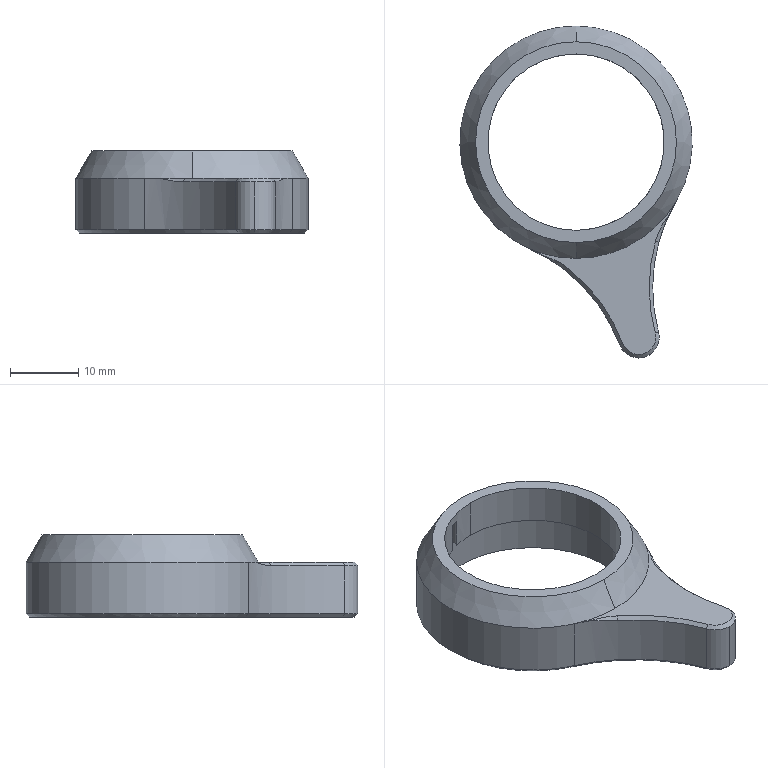Part | SolidWorks | features BaseBody 1 | 1 solid | 35 faces | box 34 x 48.563 x 12 mm | volume 4249 mm3 | cone 16 | cylinder 14 | plane 5 | commonest cylinder face diameters 2.5 x3 29.5 x3 6 x2 25.8 x2 34 x2 50 x2
STEP:
#1=CARTESIAN_POINT('',(599.943,-176.052,243.045));
#2=VERTEX_POINT('',#1);
#3=CARTESIAN_POINT('',(593.042,-208.588,243.045));
#4=VERTEX_POINT('',#3);
#5=CARTESIAN_POINT('',(599.943,-193.052,243.045));
#6=DIRECTION('',(0.000000001,-0.000000003,1.));
#7=DIRECTION('',(0.3057,-0.9521,-0.000000003));
#8=AXIS2_PLACEMENT_3D('',#5,#6,#7);
#9=CIRCLE('',#8,17.);
#10=EDGE_CURVE('',#2,#4,#9,.T.);
#11=ORIENTED_EDGE('',*,*,#10,.F.);
#12=CARTESIAN_POINT('',(599.943,-176.052,235.545));
#13=VERTEX_POINT('',#12);
#14=CARTESIAN_POINT('',(599.943,-176.052,243.045));
#15=DIRECTION('',(-0.000000001,0.000000003,-1.));
#16=VECTOR('',#15,1000.);
#17=LINE('',#14,#16);
#18=EDGE_CURVE('',#2,#13,#17,.T.);
#19=ORIENTED_EDGE('',*,*,#18,.T.);
#20=CARTESIAN_POINT('',(593.042,-208.588,235.545));
#21=VERTEX_POINT('',#20);
#22=CARTESIAN_POINT('',(599.943,-193.052,235.545));
#23=DIRECTION('',(-0.000000001,0.000000003,-1.));
#24=DIRECTION('',(0.3057,-0.9521,-0.000000003));
#25=AXIS2_PLACEMENT_3D('',#22,#23,#24);
#26=CIRCLE('',#25,17.);
#27=EDGE_CURVE('',#21,#13,#26,.T.);
#28=ORIENTED_EDGE('',*,*,#27,.F.);
#29=CARTESIAN_POINT('',(593.042,-208.588,239.295));
#30=DIRECTION('',(-0.000000001,0.000000003,-1.));
#31=VECTOR('',#30,1000.);
#32=LINE('',#29,#31);
#33=EDGE_CURVE('',#4,#21,#32,.T.);
#34=ORIENTED_EDGE('',*,*,#33,.F.);
#35=EDGE_LOOP('',(#11,#19,#28,#34));
#36=FACE_OUTER_BOUND('',#35,.T.);
#37=CARTESIAN_POINT('',(599.943,-193.052,243.045));
#38=DIRECTION('',(-0.000000001,0.000000003,-1.));
#39=DIRECTION('',(0.,1.,0.000000003));
#40=AXIS2_PLACEMENT_3D('',#37,#38,#39);
#41=CYLINDRICAL_SURFACE('',#40,17.);
#42=ADVANCED_FACE('',(#36),#41,.T.);
#43=CARTESIAN_POINT('',(599.943,-207.742,247.045));
#44=VERTEX_POINT('',#43);
#45=CARTESIAN_POINT('',(599.943,-178.361,247.045));
#46=VERTEX_POINT('',#45);
#47=CARTESIAN_POINT('',(599.943,-193.052,247.045));
#48=DIRECTION('',(0.000000001,-0.000000003,1.));
#49=DIRECTION('',(0.,1.,0.000000003));
#50=AXIS2_PLACEMENT_3D('',#47,#48,#49);
#51=CIRCLE('',#50,14.691);
#52=EDGE_CURVE('',#44,#46,#51,.T.);
#53=ORIENTED_EDGE('',*,*,#52,.F.);
#54=CARTESIAN_POINT('',(599.943,-210.052,243.045));
#55=VERTEX_POINT('',#54);
#56=CARTESIAN_POINT('',(599.943,-207.742,247.045));
#57=DIRECTION('',(-0.000000001,-0.5,-0.866));
#58=VECTOR('',#57,1000.);
#59=LINE('',#56,#58);
#60=EDGE_CURVE('',#44,#55,#59,.T.);
#61=ORIENTED_EDGE('',*,*,#60,.T.);
#62=CARTESIAN_POINT('',(614.599,-201.666,243.045));
#63=VERTEX_POINT('',#62);
#64=CARTESIAN_POINT('',(599.943,-193.052,243.045));
#65=DIRECTION('',(-0.000000001,0.000000003,-1.));
#66=DIRECTION('',(0.,1.,0.000000003));
#67=AXIS2_PLACEMENT_3D('',#64,#65,#66);
#68=CIRCLE('',#67,17.);
#69=EDGE_CURVE('',#63,#55,#68,.T.);
#70=ORIENTED_EDGE('',*,*,#69,.F.);
#71=CARTESIAN_POINT('',(599.943,-193.052,243.045));
#72=DIRECTION('',(0.000000001,-0.000000003,1.));
#73=DIRECTION('',(0.3057,-0.9521,-0.000000003));
#74=AXIS2_PLACEMENT_3D('',#71,#72,#73);
#75=CIRCLE('',#74,17.);
#76=EDGE_CURVE('',#63,#2,#75,.T.);
#77=ORIENTED_EDGE('',*,*,#76,.T.);
#78=CARTESIAN_POINT('',(599.943,-178.361,247.045));
#79=DIRECTION('',(-0.000000001,0.5,-0.866));
#80=VECTOR('',#79,1000.);
#81=LINE('',#78,#80);
#82=EDGE_CURVE('',#46,#2,#81,.T.);
#83=ORIENTED_EDGE('',*,*,#82,.F.);
#84=EDGE_LOOP('',(#53,#61,#70,#77,#83));
#85=FACE_OUTER_BOUND('',#84,.T.);
#86=CARTESIAN_POINT('',(599.943,-193.052,247.045));
#87=DIRECTION('',(-0.000000001,0.000000003,-1.));
#88=DIRECTION('',(0.,1.,0.000000003));
#89=AXIS2_PLACEMENT_3D('',#86,#87,#88);
#90=CONICAL_SURFACE('',#89,14.691,0.5236);
#91=ADVANCED_FACE('',(#85),#90,.T.);
#92=CARTESIAN_POINT('',(609.115,-224.615,235.545));
#93=VERTEX_POINT('',#92);
#94=CARTESIAN_POINT('',(606.305,-222.667,235.545));
#95=VERTEX_POINT('',#94);
#96=CARTESIAN_POINT('',(609.115,-221.615,235.545));
#97=DIRECTION('',(-0.000000001,0.000000003,-1.));
#98=DIRECTION('',(0.3057,-0.9521,-0.000000003));
#99=AXIS2_PLACEMENT_3D('',#96,#97,#98);
#100=CIRCLE('',#99,3.);
#101=EDGE_CURVE('',#93,#95,#100,.T.);
#102=ORIENTED_EDGE('',*,*,#101,.F.);
#103=CARTESIAN_POINT('',(609.115,-224.615,242.545));
#104=VERTEX_POINT('',#103);
#105=CARTESIAN_POINT('',(609.115,-224.615,235.545));
#106=DIRECTION('',(0.000000001,-0.000000003,1.));
#107=VECTOR('',#106,1000.);
#108=LINE('',#105,#107);
#109=EDGE_CURVE('',#93,#104,#108,.T.);
#110=ORIENTED_EDGE('',*,*,#109,.T.);
#111=CARTESIAN_POINT('',(606.305,-222.667,242.545));
#112=VERTEX_POINT('',#111);
#113=CARTESIAN_POINT('',(609.115,-221.615,242.545));
#114=DIRECTION('',(0.000000001,-0.000000003,1.));
#115=DIRECTION('',(0.3057,-0.9521,-0.000000003));
#116=AXIS2_PLACEMENT_3D('',#113,#114,#115);
#117=CIRCLE('',#116,3.);
#118=EDGE_CURVE('',#112,#104,#117,.T.);
#119=ORIENTED_EDGE('',*,*,#118,.F.);
#120=CARTESIAN_POINT('',(606.305,-222.667,239.295));
#121=DIRECTION('',(0.000000001,-0.000000003,1.));
#122=VECTOR('',#121,1000.);
#123=LINE('',#120,#122);
#124=EDGE_CURVE('',#95,#112,#123,.T.);
#125=ORIENTED_EDGE('',*,*,#124,.F.);
#126=EDGE_LOOP('',(#102,#110,#119,#125));
#127=FACE_OUTER_BOUND('',#126,.T.);
#128=CARTESIAN_POINT('',(609.115,-221.615,235.545));
#129=DIRECTION('',(0.000000001,-0.000000003,1.));
#130=DIRECTION('',(0.,-1.,-0.000000003));
#131=AXIS2_PLACEMENT_3D('',#128,#129,#130);
#132=CYLINDRICAL_SURFACE('',#131,3.);
#133=ADVANCED_FACE('',(#127),#132,.T.);
#134=CARTESIAN_POINT('',(599.943,-207.802,235.045));
#135=VERTEX_POINT('',#134);
#136=CARTESIAN_POINT('',(603.545,-207.355,235.045));
#137=VERTEX_POINT('',#136);
#138=CARTESIAN_POINT('',(599.943,-193.052,235.045));
#139=DIRECTION('',(0.000000001,-0.000000003,1.));
#140=DIRECTION('',(0.,-1.,-0.000000003));
#141=AXIS2_PLACEMENT_3D('',#138,#139,#140);
#142=CIRCLE('',#141,14.75);
#143=EDGE_CURVE('',#135,#137,#142,.T.);
#144=ORIENTED_EDGE('',*,*,#143,.F.);
#145=CARTESIAN_POINT('',(599.943,-207.802,241.245));
#146=VERTEX_POINT('',#145);
#147=CARTESIAN_POINT('',(599.943,-207.802,235.045));
#148=DIRECTION('',(0.000000001,-0.000000003,1.));
#149=VECTOR('',#148,1000.);
#150=LINE('',#147,#149);
#151=EDGE_CURVE('',#135,#146,#150,.T.);
#152=ORIENTED_EDGE('',*,*,#151,.T.);
#153=CARTESIAN_POINT('',(603.545,-207.355,241.245));
#154=VERTEX_POINT('',#153);
#155=CARTESIAN_POINT('',(599.943,-193.052,241.245));
#156=DIRECTION('',(0.000000001,-0.000000003,1.));
#157=DIRECTION('',(0.,-1.,-0.000000003));
#158=AXIS2_PLACEMENT_3D('',#155,#156,#157);
#159=CIRCLE('',#158,14.75);
#160=EDGE_CURVE('',#146,#154,#159,.T.);
#161=ORIENTED_EDGE('',*,*,#160,.T.);
#162=CARTESIAN_POINT('',(603.545,-207.355,238.145));
#163=DIRECTION('',(-0.000000001,0.000000003,-1.));
#164=VECTOR('',#163,1000.);
#165=LINE('',#162,#164);
#166=EDGE_CURVE('',#154,#137,#165,.T.);
#167=ORIENTED_EDGE('',*,*,#166,.T.);
#168=EDGE_LOOP('',(#144,#152,#161,#167));
#169=FACE_OUTER_BOUND('',#168,.T.);
#170=CARTESIAN_POINT('',(599.943,-193.052,235.045));
#171=DIRECTION('',(0.000000001,-0.000000003,1.));
#172=DIRECTION('',(0.,-1.,-0.000000003));
#173=AXIS2_PLACEMENT_3D('',#170,#171,#172);
#174=CYLINDRICAL_SURFACE('',#173,14.75);
#175=ADVANCED_FACE('',(#169),#174,.F.);
#176=CARTESIAN_POINT('',(609.115,-224.115,235.045));
#177=VERTEX_POINT('',#176);
#178=CARTESIAN_POINT('',(606.774,-222.492,235.045));
#179=VERTEX_POINT('',#178);
#180=CARTESIAN_POINT('',(609.115,-221.615,235.045));
#181=DIRECTION('',(-0.000000001,0.000000003,-1.));
#182=DIRECTION('',(0.,-1.,-0.000000003));
#183=AXIS2_PLACEMENT_3D('',#180,#181,#182);
#184=CIRCLE('',#183,2.5);
#185=EDGE_CURVE('',#177,#179,#184,.T.);
#186=ORIENTED_EDGE('',*,*,#185,.F.);
#187=CARTESIAN_POINT('',(609.115,-224.115,235.045));
#188=DIRECTION('',(0.000000001,-0.7071,0.7071));
#189=VECTOR('',#188,1000.);
#190=LINE('',#187,#189);
#191=EDGE_CURVE('',#177,#93,#190,.T.);
#192=ORIENTED_EDGE('',*,*,#191,.T.);
#193=ORIENTED_EDGE('',*,*,#101,.T.);
#194=CARTESIAN_POINT('',(606.539,-222.58,235.295));
#195=DIRECTION('',(-0.6622,-0.248,0.7071));
#196=VECTOR('',#195,1000.);
#197=LINE('',#194,#196);
#198=EDGE_CURVE('',#179,#95,#197,.T.);
#199=ORIENTED_EDGE('',*,*,#198,.F.);
#200=EDGE_LOOP('',(#186,#192,#193,#199));
#201=FACE_OUTER_BOUND('',#200,.T.);
#202=CARTESIAN_POINT('',(609.115,-221.615,235.045));
#203=DIRECTION('',(0.000000001,-0.000000003,1.));
#204=DIRECTION('',(0.,-1.,-0.000000003));
#205=AXIS2_PLACEMENT_3D('',#202,#203,#204);
#206=CONICAL_SURFACE('',#205,2.5,0.7854);
#207=ADVANCED_FACE('',(#201),#206,.T.);
#208=CARTESIAN_POINT('',(599.943,-180.152,247.045));
#209=VERTEX_POINT('',#208);
#210=CARTESIAN_POINT('',(599.943,-205.952,247.045));
#211=VERTEX_POINT('',#210);
#212=CARTESIAN_POINT('',(599.943,-193.052,247.045));
#213=DIRECTION('',(0.000000001,-0.000000003,1.));
#214=DIRECTION('',(0.,1.,0.000000003));
#215=AXIS2_PLACEMENT_3D('',#212,#213,#214);
#216=CIRCLE('',#215,12.9);
#217=EDGE_CURVE('',#209,#211,#216,.T.);
#218=ORIENTED_EDGE('',*,*,#217,.T.);
#219=CARTESIAN_POINT('',(599.943,-205.952,241.245));
#220=VERTEX_POINT('',#219);
#221=CARTESIAN_POINT('',(599.943,-205.952,247.045));
#222=DIRECTION('',(-0.000000001,0.000000003,-1.));
#223=VECTOR('',#222,1000.);
#224=LINE('',#221,#223);
#225=EDGE_CURVE('',#211,#220,#224,.T.);
#226=ORIENTED_EDGE('',*,*,#225,.T.);
#227=CARTESIAN_POINT('',(595.317,-181.009,241.245));
#228=VERTEX_POINT('',#227);
#229=CARTESIAN_POINT('',(599.943,-193.052,241.245));
#230=DIRECTION('',(-0.000000001,0.000000003,-1.));
#231=DIRECTION('',(0.,1.,0.000000003));
#232=AXIS2_PLACEMENT_3D('',#229,#230,#231);
#233=CIRCLE('',#232,12.9);
#234=EDGE_CURVE('',#220,#228,#233,.T.);
#235=ORIENTED_EDGE('',*,*,#234,.T.);
#236=CARTESIAN_POINT('',(595.317,-181.009,245.545));
#237=VERTEX_POINT('',#236);
#238=CARTESIAN_POINT('',(595.317,-181.009,244.145));
#239=DIRECTION('',(0.000000001,-0.000000003,1.));
#240=VECTOR('',#239,1000.);
#241=LINE('',#238,#240);
#242=EDGE_CURVE('',#228,#237,#241,.T.);
#243=ORIENTED_EDGE('',*,*,#242,.T.);
#244=CARTESIAN_POINT('',(595.693,-180.872,245.657));
#245=VERTEX_POINT('',#244);
#246=CARTESIAN_POINT('',(595.693,-180.872,245.657));
#247=CARTESIAN_POINT('',(595.565,-180.916,245.632));
#248=CARTESIAN_POINT('',(595.439,-180.962,245.592));
#249=CARTESIAN_POINT('',(595.317,-181.009,245.545));
#250=B_SPLINE_CURVE_WITH_KNOTS('',3,(#246,#247,#248,#249),.UNSPECIFIED.,.F.,.F.,(4,4),(0.001058,0.001468),.UNSPECIFIED.);
#251=EDGE_CURVE('',#245,#237,#250,.T.);
#252=ORIENTED_EDGE('',*,*,#251,.F.);
#253=CARTESIAN_POINT('',(596.693,-180.568,245.545));
#254=VERTEX_POINT('',#253);
#255=CARTESIAN_POINT('',(596.693,-180.568,245.545));
#256=CARTESIAN_POINT('',(596.53,-180.61,245.605));
#257=CARTESIAN_POINT('',(596.366,-180.656,245.653));
#258=CARTESIAN_POINT('',(596.031,-180.758,245.698));
#259=CARTESIAN_POINT('',(595.858,-180.814,245.691));
#260=CARTESIAN_POINT('',(595.693,-180.872,245.657));
#261=B_SPLINE_CURVE_WITH_KNOTS('',3,(#255,#256,#257,#258,#259,#260),.UNSPECIFIED.,.F.,.F.,(4,2,4),(0.,0.0005289,0.001058),.UNSPECIFIED.);
#262=EDGE_CURVE('',#254,#245,#261,.T.);
#263=ORIENTED_EDGE('',*,*,#262,.F.);
#264=CARTESIAN_POINT('',(596.693,-180.568,241.245));
#265=VERTEX_POINT('',#264);
#266=CARTESIAN_POINT('',(596.693,-180.568,244.145));
#267=DIRECTION('',(-0.000000001,0.000000003,-1.));
#268=VECTOR('',#267,1000.);
#269=LINE('',#266,#268);
#270=EDGE_CURVE('',#254,#265,#269,.T.);
#271=ORIENTED_EDGE('',*,*,#270,.T.);
#272=CARTESIAN_POINT('',(599.943,-180.152,241.245));
#273=VERTEX_POINT('',#272);
#274=CARTESIAN_POINT('',(599.943,-193.052,241.245));
#275=DIRECTION('',(-0.000000001,0.000000003,-1.));
#276=DIRECTION('',(0.,1.,0.000000003));
#277=AXIS2_PLACEMENT_3D('',#274,#275,#276);
#278=CIRCLE('',#277,12.9);
#279=EDGE_CURVE('',#265,#273,#278,.T.);
#280=ORIENTED_EDGE('',*,*,#279,.T.);
#281=CARTESIAN_POINT('',(599.943,-180.152,247.045));
#282=DIRECTION('',(-0.000000001,0.000000003,-1.));
#283=VECTOR('',#282,1000.);
#284=LINE('',#281,#283);
#285=EDGE_CURVE('',#209,#273,#284,.T.);
#286=ORIENTED_EDGE('',*,*,#285,.F.);
#287=EDGE_LOOP('',(#218,#226,#235,#243,#252,#263,#271,#280,#286));
#288=FACE_OUTER_BOUND('',#287,.T.);
#289=CARTESIAN_POINT('',(599.943,-193.052,247.045));
#290=DIRECTION('',(-0.000000001,0.000000003,-1.));
#291=DIRECTION('',(0.,1.,0.000000003));
#292=AXIS2_PLACEMENT_3D('',#289,#290,#291);
#293=CYLINDRICAL_SURFACE('',#292,12.9);
#294=ADVANCED_FACE('',(#288),#293,.F.);
#295=CARTESIAN_POINT('',(595.693,-178.567,245.545));
#296=VERTEX_POINT('',#295);
#297=CARTESIAN_POINT('',(595.693,-179.817,245.545));
#298=DIRECTION('',(0.000000001,-0.000000003,1.));
#299=DIRECTION('',(0.3057,-0.9521,-0.000000003));
#300=AXIS2_PLACEMENT_3D('',#297,#298,#299);
#301=CIRCLE('',#300,1.25);
#302=EDGE_CURVE('',#254,#296,#301,.T.);
#303=ORIENTED_EDGE('',*,*,#302,.T.);
#304=CARTESIAN_POINT('',(595.693,-178.567,235.045));
#305=VERTEX_POINT('',#304);
#306=CARTESIAN_POINT('',(595.693,-178.567,245.545));
#307=DIRECTION('',(-0.000000001,0.000000003,-1.));
#308=VECTOR('',#307,1000.);
#309=LINE('',#306,#308);
#310=EDGE_CURVE('',#296,#305,#309,.T.);
#311=ORIENTED_EDGE('',*,*,#310,.T.);
#312=CARTESIAN_POINT('',(596.341,-178.748,235.045));
#313=VERTEX_POINT('',#312);
#314=CARTESIAN_POINT('',(595.693,-179.817,235.045));
#315=DIRECTION('',(-0.000000001,0.000000003,-1.));
#316=DIRECTION('',(0.,1.,0.000000003));
#317=AXIS2_PLACEMENT_3D('',#314,#315,#316);
#318=CIRCLE('',#317,1.25);
#319=EDGE_CURVE('',#305,#313,#318,.T.);
#320=ORIENTED_EDGE('',*,*,#319,.T.);
#321=CARTESIAN_POINT('',(596.341,-178.748,241.245));
#322=VERTEX_POINT('',#321);
#323=CARTESIAN_POINT('',(596.341,-178.748,238.145));
#324=DIRECTION('',(-0.000000001,0.000000003,-1.));
#325=VECTOR('',#324,1000.);
#326=LINE('',#323,#325);
#327=EDGE_CURVE('',#322,#313,#326,.T.);
#328=ORIENTED_EDGE('',*,*,#327,.F.);
#329=CARTESIAN_POINT('',(595.693,-179.817,241.245));
#330=DIRECTION('',(-0.000000001,0.000000003,-1.));
#331=DIRECTION('',(0.,1.,0.000000003));
#332=AXIS2_PLACEMENT_3D('',#329,#330,#331);
#333=CIRCLE('',#332,1.25);
#334=EDGE_CURVE('',#322,#265,#333,.T.);
#335=ORIENTED_EDGE('',*,*,#334,.T.);
#336=ORIENTED_EDGE('',*,*,#270,.F.);
#337=EDGE_LOOP('',(#303,#311,#320,#328,#335,#336));
#338=FACE_OUTER_BOUND('',#337,.T.);
#339=CARTESIAN_POINT('',(595.693,-179.817,245.545));
#340=DIRECTION('',(-0.000000001,0.000000003,-1.));
#341=DIRECTION('',(0.,1.,0.000000003));
#342=AXIS2_PLACEMENT_3D('',#339,#340,#341);
#343=CYLINDRICAL_SURFACE('',#342,1.25);
#344=ADVANCED_FACE('',(#338),#343,.F.);
#345=CARTESIAN_POINT('',(604.192,-206.286,246.266));
#346=VERTEX_POINT('',#345);
#347=CARTESIAN_POINT('',(604.192,-205.231,245.657));
#348=VERTEX_POINT('',#347);
#349=CARTESIAN_POINT('',(604.192,-206.286,246.266));
#350=DIRECTION('',(0.,0.866,-0.5));
#351=VECTOR('',#350,1000.);
#352=LINE('',#349,#351);
#353=EDGE_CURVE('',#346,#348,#352,.T.);
#354=ORIENTED_EDGE('',*,*,#353,.F.);
#355=CARTESIAN_POINT('',(604.192,-207.536,245.545));
#356=VERTEX_POINT('',#355);
#357=CARTESIAN_POINT('',(604.192,-206.286,246.266));
#358=DIRECTION('',(0.,-0.866,-0.5));
#359=VECTOR('',#358,1000.);
#360=LINE('',#357,#359);
#361=EDGE_CURVE('',#346,#356,#360,.T.);
#362=ORIENTED_EDGE('',*,*,#361,.T.);
#363=CARTESIAN_POINT('',(603.193,-205.535,245.545));
#364=VERTEX_POINT('',#363);
#365=CARTESIAN_POINT('',(604.192,-206.286,245.545));
#366=DIRECTION('',(0.000000001,-0.000000003,1.));
#367=DIRECTION('',(0.3057,-0.9521,-0.000000003));
#368=AXIS2_PLACEMENT_3D('',#365,#366,#367);
#369=CIRCLE('',#368,1.25);
#370=EDGE_CURVE('',#364,#356,#369,.T.);
#371=ORIENTED_EDGE('',*,*,#370,.F.);
#372=CARTESIAN_POINT('',(603.193,-205.535,245.545));
#373=CARTESIAN_POINT('',(603.355,-205.493,245.605));
#374=CARTESIAN_POINT('',(603.519,-205.447,245.653));
#375=CARTESIAN_POINT('',(603.855,-205.345,245.698));
#376=CARTESIAN_POINT('',(604.028,-205.289,245.691));
#377=CARTESIAN_POINT('',(604.192,-205.231,245.657));
#378=B_SPLINE_CURVE_WITH_KNOTS('',3,(#372,#373,#374,#375,#376,#377),.UNSPECIFIED.,.F.,.F.,(4,2,4),(-0.0007426,-0.0002096,0.0003234),.UNSPECIFIED.);
#379=EDGE_CURVE('',#364,#348,#378,.T.);
#380=ORIENTED_EDGE('',*,*,#379,.T.);
#381=EDGE_LOOP('',(#354,#362,#371,#380));
#382=FACE_OUTER_BOUND('',#381,.T.);
#383=CARTESIAN_POINT('',(604.192,-206.286,-753.734));
#384=DIRECTION('',(-0.000000001,0.000000003,-1.));
#385=DIRECTION('',(0.,1.,0.000000003));
#386=AXIS2_PLACEMENT_3D('',#383,#384,#385);
#387=CONICAL_SURFACE('',#386,1732.051,1.047);
#388=ADVANCED_FACE('',(#382),#387,.F.);
#389=CARTESIAN_POINT('',(595.693,-179.817,246.266));
#390=VERTEX_POINT('',#389);
#391=CARTESIAN_POINT('',(595.693,-179.817,246.266));
#392=DIRECTION('',(0.,0.866,-0.5));
#393=VECTOR('',#392,1000.);
#394=LINE('',#391,#393);
#395=EDGE_CURVE('',#390,#296,#394,.T.);
#396=ORIENTED_EDGE('',*,*,#395,.F.);
#397=CARTESIAN_POINT('',(595.693,-179.817,246.266));
#398=DIRECTION('',(0.,-0.866,-0.5));
#399=VECTOR('',#398,1000.);
#400=LINE('',#397,#399);
#401=EDGE_CURVE('',#390,#245,#400,.T.);
#402=ORIENTED_EDGE('',*,*,#401,.T.);
#403=ORIENTED_EDGE('',*,*,#251,.T.);
#404=CARTESIAN_POINT('',(595.693,-179.817,245.545));
#405=DIRECTION('',(0.000000001,-0.000000003,1.));
#406=DIRECTION('',(0.3057,-0.9521,-0.000000003));
#407=AXIS2_PLACEMENT_3D('',#404,#405,#406);
#408=CIRCLE('',#407,1.25);
#409=EDGE_CURVE('',#296,#237,#408,.T.);
#410=ORIENTED_EDGE('',*,*,#409,.F.);
#411=EDGE_LOOP('',(#396,#402,#403,#410));
#412=FACE_OUTER_BOUND('',#411,.T.);
#413=CARTESIAN_POINT('',(595.693,-179.817,-753.734));
#414=DIRECTION('',(-0.000000001,0.000000003,-1.));
#415=DIRECTION('',(0.,1.,0.000000003));
#416=AXIS2_PLACEMENT_3D('',#413,#414,#415);
#417=CONICAL_SURFACE('',#416,1732.051,1.047);
#418=ADVANCED_FACE('',(#412),#417,.F.);
#419=ORIENTED_EDGE('',*,*,#18,.F.);
#420=ORIENTED_EDGE('',*,*,#76,.F.);
#421=CARTESIAN_POINT('',(614.599,-201.666,235.545));
#422=VERTEX_POINT('',#421);
#423=CARTESIAN_POINT('',(614.599,-201.666,239.295));
#424=DIRECTION('',(0.000000001,-0.000000003,1.));
#425=VECTOR('',#424,1000.);
#426=LINE('',#423,#425);
#427=EDGE_CURVE('',#422,#63,#426,.T.);
#428=ORIENTED_EDGE('',*,*,#427,.F.);
#429=CARTESIAN_POINT('',(599.943,-193.052,235.545));
#430=DIRECTION('',(-0.000000001,0.000000003,-1.));
#431=DIRECTION('',(0.3057,-0.9521,-0.000000003));
#432=AXIS2_PLACEMENT_3D('',#429,#430,#431);
#433=CIRCLE('',#432,17.);
#434=EDGE_CURVE('',#13,#422,#433,.T.);
#435=ORIENTED_EDGE('',*,*,#434,.F.);
#436=EDGE_LOOP('',(#419,#420,#428,#435));
#437=FACE_OUTER_BOUND('',#436,.T.);
#438=CARTESIAN_POINT('',(599.943,-193.052,243.045));
#439=DIRECTION('',(-0.000000001,0.000000003,-1.));
#440=DIRECTION('',(0.,1.,0.000000003));
#441=AXIS2_PLACEMENT_3D('',#438,#439,#440);
#442=CYLINDRICAL_SURFACE('',#441,17.);
#443=ADVANCED_FACE('',(#437),#442,.T.);
#444=CARTESIAN_POINT('',(593.245,-208.131,235.045));
#445=VERTEX_POINT('',#444);
#446=CARTESIAN_POINT('',(614.168,-201.412,235.045));
#447=VERTEX_POINT('',#446);
#448=CARTESIAN_POINT('',(599.943,-193.052,235.045));
#449=DIRECTION('',(-0.000000001,0.000000003,-1.));
#450=DIRECTION('',(0.,-1.,-0.000000003));
#451=AXIS2_PLACEMENT_3D('',#448,#449,#450);
#452=CIRCLE('',#451,16.5);
#453=EDGE_CURVE('',#445,#447,#452,.T.);
#454=ORIENTED_EDGE('',*,*,#453,.F.);
#455=CARTESIAN_POINT('',(593.143,-208.359,235.295));
#456=DIRECTION('',(0.287,0.6462,-0.7071));
#457=VECTOR('',#456,1000.);
#458=LINE('',#455,#457);
#459=EDGE_CURVE('',#21,#445,#458,.T.);
#460=ORIENTED_EDGE('',*,*,#459,.F.);
#461=ORIENTED_EDGE('',*,*,#27,.T.);
#462=ORIENTED_EDGE('',*,*,#434,.T.);
#463=CARTESIAN_POINT('',(614.383,-201.539,235.295));
#464=DIRECTION('',(0.6096,-0.3583,0.7071));
#465=VECTOR('',#464,1000.);
#466=LINE('',#463,#465);
#467=EDGE_CURVE('',#447,#422,#466,.T.);
#468=ORIENTED_EDGE('',*,*,#467,.F.);
#469=EDGE_LOOP('',(#454,#460,#461,#462,#468));
#470=FACE_OUTER_BOUND('',#469,.T.);
#471=CARTESIAN_POINT('',(599.943,-193.052,235.545));
#472=DIRECTION('',(0.000000001,-0.000000003,1.));
#473=DIRECTION('',(0.,-1.,-0.000000003));
#474=AXIS2_PLACEMENT_3D('',#471,#472,#473);
#475=CONICAL_SURFACE('',#474,17.,0.7854);
#476=ADVANCED_FACE('',(#470),#475,.T.);
#477=CARTESIAN_POINT('',(598.569,-211.96,242.545));
#478=VERTEX_POINT('',#477);
#479=CARTESIAN_POINT('',(582.893,-231.435,242.545));
#480=DIRECTION('',(0.000000001,-0.000000003,1.));
#481=DIRECTION('',(0.3057,-0.9521,-0.000000003));
#482=AXIS2_PLACEMENT_3D('',#479,#480,#481);
#483=CIRCLE('',#482,25.);
#484=EDGE_CURVE('',#112,#478,#483,.T.);
#485=ORIENTED_EDGE('',*,*,#484,.T.);
#486=CARTESIAN_POINT('',(595.292,-209.727,243.045));
#487=VERTEX_POINT('',#486);
#488=CARTESIAN_POINT('',(598.569,-211.96,242.545));
#489=CARTESIAN_POINT('',(597.52,-211.116,242.545));
#490=CARTESIAN_POINT('',(596.427,-210.375,242.724));
#491=CARTESIAN_POINT('',(595.292,-209.727,243.045));
#492=B_SPLINE_CURVE_WITH_KNOTS('',3,(#488,#489,#490,#491),.UNSPECIFIED.,.F.,.F.,(4,4),(0.,0.003997),.UNSPECIFIED.);
#493=EDGE_CURVE('',#478,#487,#492,.T.);
#494=ORIENTED_EDGE('',*,*,#493,.T.);
#495=CARTESIAN_POINT('',(582.893,-231.435,243.045));
#496=DIRECTION('',(0.000000001,-0.000000003,1.));
#497=DIRECTION('',(0.,-1.,-0.000000003));
#498=AXIS2_PLACEMENT_3D('',#495,#496,#497);
#499=CIRCLE('',#498,25.);
#500=EDGE_CURVE('',#487,#4,#499,.T.);
#501=ORIENTED_EDGE('',*,*,#500,.T.);
#502=ORIENTED_EDGE('',*,*,#33,.T.);
#503=CARTESIAN_POINT('',(582.893,-231.435,235.545));
#504=DIRECTION('',(-0.000000001,0.000000003,-1.));
#505=DIRECTION('',(0.3057,-0.9521,-0.000000003));
#506=AXIS2_PLACEMENT_3D('',#503,#504,#505);
#507=CIRCLE('',#506,25.);
#508=EDGE_CURVE('',#21,#95,#507,.T.);
#509=ORIENTED_EDGE('',*,*,#508,.T.);
#510=ORIENTED_EDGE('',*,*,#124,.T.);
#511=EDGE_LOOP('',(#485,#494,#501,#502,#509,#510));
#512=FACE_OUTER_BOUND('',#511,.T.);
#513=CARTESIAN_POINT('',(582.893,-231.435,235.545));
#514=DIRECTION('',(0.000000001,-0.000000003,1.));
#515=DIRECTION('',(0.,-1.,-0.000000003));
#516=AXIS2_PLACEMENT_3D('',#513,#514,#515);
#517=CYLINDRICAL_SURFACE('',#516,25.);
#518=ADVANCED_FACE('',(#512),#517,.F.);
#519=ORIENTED_EDGE('',*,*,#60,.F.);
#520=CARTESIAN_POINT('',(599.943,-193.052,247.045));
#521=DIRECTION('',(0.000000001,-0.000000003,1.));
#522=DIRECTION('',(0.,1.,0.000000003));
#523=AXIS2_PLACEMENT_3D('',#520,#521,#522);
#524=CIRCLE('',#523,14.691);
#525=EDGE_CURVE('',#46,#44,#524,.T.);
#526=ORIENTED_EDGE('',*,*,#525,.F.);
#527=ORIENTED_EDGE('',*,*,#82,.T.);
#528=ORIENTED_EDGE('',*,*,#10,.T.);
#529=CARTESIAN_POINT('',(599.943,-193.052,243.045));
#530=DIRECTION('',(-0.000000001,0.000000003,-1.));
#531=DIRECTION('',(0.,1.,0.000000003));
#532=AXIS2_PLACEMENT_3D('',#529,#530,#531);
#533=CIRCLE('',#532,17.);
#534=EDGE_CURVE('',#55,#4,#533,.T.);
#535=ORIENTED_EDGE('',*,*,#534,.F.);
#536=EDGE_LOOP('',(#519,#526,#527,#528,#535));
#537=FACE_OUTER_BOUND('',#536,.T.);
#538=CARTESIAN_POINT('',(599.943,-193.052,247.045));
#539=DIRECTION('',(-0.000000001,0.000000003,-1.));
#540=DIRECTION('',(0.,1.,0.000000003));
#541=AXIS2_PLACEMENT_3D('',#538,#539,#540);
#542=CONICAL_SURFACE('',#541,14.691,0.5236);
#543=ADVANCED_FACE('',(#537),#542,.T.);
#544=CARTESIAN_POINT('',(612.012,-220.835,235.545));
#545=VERTEX_POINT('',#544);
#546=CARTESIAN_POINT('',(636.151,-214.334,235.545));
#547=DIRECTION('',(-0.000000001,0.000000003,-1.));
#548=DIRECTION('',(0.3057,-0.9521,-0.000000003));
#549=AXIS2_PLACEMENT_3D('',#546,#547,#548);
#550=CIRCLE('',#549,25.);
#551=EDGE_CURVE('',#545,#422,#550,.T.);
#552=ORIENTED_EDGE('',*,*,#551,.T.);
#553=ORIENTED_EDGE('',*,*,#427,.T.);
#554=CARTESIAN_POINT('',(613.432,-203.902,243.045));
#555=VERTEX_POINT('',#554);
#556=CARTESIAN_POINT('',(636.151,-214.334,243.045));
#557=DIRECTION('',(0.000000001,-0.000000003,1.));
#558=DIRECTION('',(0.,-1.,-0.000000003));
#559=AXIS2_PLACEMENT_3D('',#556,#557,#558);
#560=CIRCLE('',#559,25.);
#561=EDGE_CURVE('',#63,#555,#560,.T.);
#562=ORIENTED_EDGE('',*,*,#561,.T.);
#563=CARTESIAN_POINT('',(612.068,-207.626,242.545));
#564=VERTEX_POINT('',#563);
#565=CARTESIAN_POINT('',(613.432,-203.902,243.045));
#566=CARTESIAN_POINT('',(612.887,-205.089,242.724));
#567=CARTESIAN_POINT('',(612.43,-206.328,242.545));
#568=CARTESIAN_POINT('',(612.068,-207.626,242.545));
#569=B_SPLINE_CURVE_WITH_KNOTS('',3,(#565,#566,#567,#568),.UNSPECIFIED.,.F.,.F.,(4,4),(0.,0.003997),.UNSPECIFIED.);
#570=EDGE_CURVE('',#555,#564,#569,.T.);
#571=ORIENTED_EDGE('',*,*,#570,.T.);
#572=CARTESIAN_POINT('',(612.012,-220.835,242.545));
#573=VERTEX_POINT('',#572);
#574=CARTESIAN_POINT('',(636.151,-214.334,242.545));
#575=DIRECTION('',(0.000000001,-0.000000003,1.));
#576=DIRECTION('',(0.3057,-0.9521,-0.000000003));
#577=AXIS2_PLACEMENT_3D('',#574,#575,#576);
#578=CIRCLE('',#577,25.);
#579=EDGE_CURVE('',#564,#573,#578,.T.);
#580=ORIENTED_EDGE('',*,*,#579,.T.);
#581=CARTESIAN_POINT('',(612.012,-220.835,239.295));
#582=DIRECTION('',(-0.000000001,0.000000003,-1.));
#583=VECTOR('',#582,1000.);
#584=LINE('',#581,#583);
#585=EDGE_CURVE('',#573,#545,#584,.T.);
#586=ORIENTED_EDGE('',*,*,#585,.T.);
#587=EDGE_LOOP('',(#552,#553,#562,#571,#580,#586));
#588=FACE_OUTER_BOUND('',#587,.T.);
#589=CARTESIAN_POINT('',(636.151,-214.334,235.545));
#590=DIRECTION('',(0.000000001,-0.000000003,1.));
#591=DIRECTION('',(0.,-1.,-0.000000003));
#592=AXIS2_PLACEMENT_3D('',#589,#590,#591);
#593=CYLINDRICAL_SURFACE('',#592,25.);
#594=ADVANCED_FACE('',(#588),#593,.F.);
#595=CARTESIAN_POINT('',(605.342,-206.778,235.045));
#596=VERTEX_POINT('',#595);
#597=CARTESIAN_POINT('',(604.192,-206.286,235.045));
#598=DIRECTION('',(-0.000000001,0.000000003,-1.));
#599=DIRECTION('',(0.,1.,0.000000003));
#600=AXIS2_PLACEMENT_3D('',#597,#598,#599);
#601=CIRCLE('',#600,1.25);
#602=EDGE_CURVE('',#596,#137,#601,.T.);
#603=ORIENTED_EDGE('',*,*,#602,.F.);
#604=CARTESIAN_POINT('',(599.943,-193.052,235.045));
#605=DIRECTION('',(0.000000001,-0.000000003,1.));
#606=DIRECTION('',(0.,-1.,-0.000000003));
#607=AXIS2_PLACEMENT_3D('',#604,#605,#606);
#608=CIRCLE('',#607,14.75);
#609=EDGE_CURVE('',#596,#313,#608,.T.);
#610=ORIENTED_EDGE('',*,*,#609,.T.);
#611=ORIENTED_EDGE('',*,*,#319,.F.);
#612=CARTESIAN_POINT('',(594.544,-179.325,235.045));
#613=VERTEX_POINT('',#612);
#614=CARTESIAN_POINT('',(595.693,-179.817,235.045));
#615=DIRECTION('',(-0.000000001,0.000000003,-1.));
#616=DIRECTION('',(0.,1.,0.000000003));
#617=AXIS2_PLACEMENT_3D('',#614,#615,#616);
#618=CIRCLE('',#617,1.25);
#619=EDGE_CURVE('',#613,#305,#618,.T.);
#620=ORIENTED_EDGE('',*,*,#619,.F.);
#621=CARTESIAN_POINT('',(599.943,-193.052,235.045));
#622=DIRECTION('',(0.000000001,-0.000000003,1.));
#623=DIRECTION('',(0.,-1.,-0.000000003));
#624=AXIS2_PLACEMENT_3D('',#621,#622,#623);
#625=CIRCLE('',#624,14.75);
#626=EDGE_CURVE('',#613,#135,#625,.T.);
#627=ORIENTED_EDGE('',*,*,#626,.T.);
#628=ORIENTED_EDGE('',*,*,#143,.T.);
#629=EDGE_LOOP('',(#603,#610,#611,#620,#627,#628));
#630=FACE_BOUND('',#629,.T.);
#631=CARTESIAN_POINT('',(611.529,-220.965,235.045));
#632=VERTEX_POINT('',#631);
#633=CARTESIAN_POINT('',(609.115,-221.615,235.045));
#634=DIRECTION('',(-0.000000001,0.000000003,-1.));
#635=DIRECTION('',(0.,-1.,-0.000000003));
#636=AXIS2_PLACEMENT_3D('',#633,#634,#635);
#637=CIRCLE('',#636,2.5);
#638=EDGE_CURVE('',#632,#177,#637,.T.);
#639=ORIENTED_EDGE('',*,*,#638,.T.);
#640=ORIENTED_EDGE('',*,*,#185,.T.);
#641=CARTESIAN_POINT('',(582.893,-231.435,235.045));
#642=DIRECTION('',(0.000000001,-0.000000003,1.));
#643=DIRECTION('',(0.,1.,0.000000003));
#644=AXIS2_PLACEMENT_3D('',#641,#642,#643);
#645=CIRCLE('',#644,25.5);
#646=EDGE_CURVE('',#179,#445,#645,.T.);
#647=ORIENTED_EDGE('',*,*,#646,.T.);
#648=ORIENTED_EDGE('',*,*,#453,.T.);
#649=CARTESIAN_POINT('',(636.151,-214.334,235.045));
#650=DIRECTION('',(0.000000001,-0.000000003,1.));
#651=DIRECTION('',(0.,1.,0.000000003));
#652=AXIS2_PLACEMENT_3D('',#649,#650,#651);
#653=CIRCLE('',#652,25.5);
#654=EDGE_CURVE('',#447,#632,#653,.T.);
#655=ORIENTED_EDGE('',*,*,#654,.T.);
#656=EDGE_LOOP('',(#639,#640,#647,#648,#655));
#657=FACE_OUTER_BOUND('',#656,.T.);
#658=CARTESIAN_POINT('',(610.946,-171.159,235.045));
#659=DIRECTION('',(-0.000000001,0.000000003,-1.));
#660=DIRECTION('',(0.3057,-0.9521,-0.000000003));
#661=AXIS2_PLACEMENT_3D('',#658,#659,#660);
#662=PLANE('',#661);
#663=ADVANCED_FACE('',(#630,#657),#662,.T.);
#664=CARTESIAN_POINT('',(598.882,-211.571,243.045));
#665=VERTEX_POINT('',#664);
#666=CARTESIAN_POINT('',(598.725,-211.767,242.793));
#667=DIRECTION('',(0.4434,0.5508,0.7071));
#668=VECTOR('',#667,1000.);
#669=LINE('',#666,#668);
#670=EDGE_CURVE('',#478,#665,#669,.T.);
#671=ORIENTED_EDGE('',*,*,#670,.T.);
#672=CARTESIAN_POINT('',(592.612,-219.361,243.045));
#673=DIRECTION('',(0.000000001,-0.000000003,1.));
#674=DIRECTION('',(0.,-1.,-0.000000003));
#675=AXIS2_PLACEMENT_3D('',#672,#673,#674);
#676=CIRCLE('',#675,10.);
#677=EDGE_CURVE('',#665,#487,#676,.T.);
#678=ORIENTED_EDGE('',*,*,#677,.T.);
#679=ORIENTED_EDGE('',*,*,#493,.F.);
#680=EDGE_LOOP('',(#671,#678,#679));
#681=FACE_OUTER_BOUND('',#680,.T.);
#682=CARTESIAN_POINT('',(592.612,-219.361,242.542));
#683=DIRECTION('',(0.000000001,-0.000000003,1.));
#684=DIRECTION('',(0.,-1.,-0.000000003));
#685=AXIS2_PLACEMENT_3D('',#682,#683,#684);
#686=CONICAL_SURFACE('',#685,9.497,0.7854);
#687=ADVANCED_FACE('',(#681),#686,.F.);
#688=CARTESIAN_POINT('',(606.774,-222.492,243.045));
#689=VERTEX_POINT('',#688);
#690=CARTESIAN_POINT('',(582.893,-231.435,243.045));
#691=DIRECTION('',(0.000000001,-0.000000003,1.));
#692=DIRECTION('',(0.,-1.,-0.000000003));
#693=AXIS2_PLACEMENT_3D('',#690,#691,#692);
#694=CIRCLE('',#693,25.5);
#695=EDGE_CURVE('',#689,#665,#694,.T.);
#696=ORIENTED_EDGE('',*,*,#695,.T.);
#697=ORIENTED_EDGE('',*,*,#670,.F.);
#698=ORIENTED_EDGE('',*,*,#484,.F.);
#699=CARTESIAN_POINT('',(606.539,-222.58,242.795));
#700=DIRECTION('',(0.6622,0.248,0.7071));
#701=VECTOR('',#700,1000.);
#702=LINE('',#699,#701);
#703=EDGE_CURVE('',#112,#689,#702,.T.);
#704=ORIENTED_EDGE('',*,*,#703,.T.);
#705=EDGE_LOOP('',(#696,#697,#698,#704));
#706=FACE_OUTER_BOUND('',#705,.T.);
#707=CARTESIAN_POINT('',(582.893,-231.435,242.545));
#708=DIRECTION('',(0.000000001,-0.000000003,1.));
#709=DIRECTION('',(0.,-1.,-0.000000003));
#710=AXIS2_PLACEMENT_3D('',#707,#708,#709);
#711=CONICAL_SURFACE('',#710,25.,0.7854);
#712=ADVANCED_FACE('',(#706),#711,.F.);
#713=ORIENTED_EDGE('',*,*,#109,.F.);
#714=CARTESIAN_POINT('',(609.115,-221.615,235.545));
#715=DIRECTION('',(-0.000000001,0.000000003,-1.));
#716=DIRECTION('',(0.3057,-0.9521,-0.000000003));
#717=AXIS2_PLACEMENT_3D('',#714,#715,#716);
#718=CIRCLE('',#717,3.);
#719=EDGE_CURVE('',#545,#93,#718,.T.);
#720=ORIENTED_EDGE('',*,*,#719,.F.);
#721=ORIENTED_EDGE('',*,*,#585,.F.);
#722=CARTESIAN_POINT('',(609.115,-221.615,242.545));
#723=DIRECTION('',(0.000000001,-0.000000003,1.));
#724=DIRECTION('',(0.3057,-0.9521,-0.000000003));
#725=AXIS2_PLACEMENT_3D('',#722,#723,#724);
#726=CIRCLE('',#725,3.);
#727=EDGE_CURVE('',#104,#573,#726,.T.);
#728=ORIENTED_EDGE('',*,*,#727,.F.);
#729=EDGE_LOOP('',(#713,#720,#721,#728));
#730=FACE_OUTER_BOUND('',#729,.T.);
#731=CARTESIAN_POINT('',(609.115,-221.615,235.545));
#732=DIRECTION('',(0.000000001,-0.000000003,1.));
#733=DIRECTION('',(0.,-1.,-0.000000003));
#734=AXIS2_PLACEMENT_3D('',#731,#732,#733);
#735=CYLINDRICAL_SURFACE('',#734,3.);
#736=ADVANCED_FACE('',(#730),#735,.T.);
#737=ORIENTED_EDGE('',*,*,#508,.F.);
#738=ORIENTED_EDGE('',*,*,#459,.T.);
#739=ORIENTED_EDGE('',*,*,#646,.F.);
#740=ORIENTED_EDGE('',*,*,#198,.T.);
#741=EDGE_LOOP('',(#737,#738,#739,#740));
#742=FACE_OUTER_BOUND('',#741,.T.);
#743=CARTESIAN_POINT('',(582.893,-231.435,235.045));
#744=DIRECTION('',(-0.000000001,0.000000003,-1.));
#745=DIRECTION('',(0.,1.,0.000000003));
#746=AXIS2_PLACEMENT_3D('',#743,#744,#745);
#747=CONICAL_SURFACE('',#746,25.5,0.7854);
#748=ADVANCED_FACE('',(#742),#747,.F.);
#749=CARTESIAN_POINT('',(611.587,-207.491,243.045));
#750=VERTEX_POINT('',#749);
#751=CARTESIAN_POINT('',(621.22,-210.175,243.045));
#752=DIRECTION('',(-0.000000001,0.000000003,-1.));
#753=DIRECTION('',(0.,-1.,-0.000000003));
#754=AXIS2_PLACEMENT_3D('',#751,#752,#753);
#755=CIRCLE('',#754,10.);
#756=EDGE_CURVE('',#750,#555,#755,.T.);
#757=ORIENTED_EDGE('',*,*,#756,.T.);
#758=ORIENTED_EDGE('',*,*,#561,.F.);
#759=ORIENTED_EDGE('',*,*,#69,.T.);
#760=ORIENTED_EDGE('',*,*,#534,.T.);
#761=ORIENTED_EDGE('',*,*,#500,.F.);
#762=ORIENTED_EDGE('',*,*,#677,.F.);
#763=ORIENTED_EDGE('',*,*,#695,.F.);
#764=CARTESIAN_POINT('',(611.529,-220.965,243.045));
#765=VERTEX_POINT('',#764);
#766=CARTESIAN_POINT('',(609.115,-221.615,243.045));
#767=DIRECTION('',(0.000000001,-0.000000003,1.));
#768=DIRECTION('',(0.,1.,0.000000003));
#769=AXIS2_PLACEMENT_3D('',#766,#767,#768);
#770=CIRCLE('',#769,2.5);
#771=EDGE_CURVE('',#689,#765,#770,.T.);
#772=ORIENTED_EDGE('',*,*,#771,.T.);
#773=CARTESIAN_POINT('',(636.151,-214.334,243.045));
#774=DIRECTION('',(-0.000000001,0.000000003,-1.));
#775=DIRECTION('',(0.,-1.,-0.000000003));
#776=AXIS2_PLACEMENT_3D('',#773,#774,#775);
#777=CIRCLE('',#776,25.5);
#778=EDGE_CURVE('',#765,#750,#777,.T.);
#779=ORIENTED_EDGE('',*,*,#778,.T.);
#780=EDGE_LOOP('',(#757,#758,#759,#760,#761,#762,#763,#772,#779));
#781=FACE_OUTER_BOUND('',#780,.T.);
#782=CARTESIAN_POINT('',(592.489,-208.349,243.045));
#783=DIRECTION('',(0.000000001,-0.000000003,1.));
#784=DIRECTION('',(0.3057,-0.9521,-0.000000003));
#785=AXIS2_PLACEMENT_3D('',#782,#783,#784);
#786=PLANE('',#785);
#787=ADVANCED_FACE('',(#781),#786,.T.);
#788=ORIENTED_EDGE('',*,*,#217,.F.);
#789=CARTESIAN_POINT('',(599.943,-193.052,247.045));
#790=DIRECTION('',(0.000000001,-0.000000003,1.));
#791=DIRECTION('',(0.,1.,0.000000003));
#792=AXIS2_PLACEMENT_3D('',#789,#790,#791);
#793=CIRCLE('',#792,12.9);
#794=EDGE_CURVE('',#211,#209,#793,.T.);
#795=ORIENTED_EDGE('',*,*,#794,.F.);
#796=EDGE_LOOP('',(#788,#795));
#797=FACE_BOUND('',#796,.T.);
#798=ORIENTED_EDGE('',*,*,#525,.T.);
#799=ORIENTED_EDGE('',*,*,#52,.T.);
#800=EDGE_LOOP('',(#798,#799));
#801=FACE_OUTER_BOUND('',#800,.T.);
#802=CARTESIAN_POINT('',(609.83,-173.83,247.045));
#803=DIRECTION('',(-0.000000001,0.000000003,-1.));
#804=DIRECTION('',(0.3057,-0.9521,-0.000000003));
#805=AXIS2_PLACEMENT_3D('',#802,#803,#804);
#806=PLANE('',#805);
#807=ADVANCED_FACE('',(#797,#801),#806,.F.);
#808=ORIENTED_EDGE('',*,*,#551,.F.);
#809=CARTESIAN_POINT('',(611.77,-220.9,235.295));
#810=DIRECTION('',(-0.6828,-0.1839,-0.7071));
#811=VECTOR('',#810,1000.);
#812=LINE('',#809,#811);
#813=EDGE_CURVE('',#545,#632,#812,.T.);
#814=ORIENTED_EDGE('',*,*,#813,.T.);
#815=ORIENTED_EDGE('',*,*,#654,.F.);
#816=ORIENTED_EDGE('',*,*,#467,.T.);
#817=EDGE_LOOP('',(#808,#814,#815,#816));
#818=FACE_OUTER_BOUND('',#817,.T.);
#819=CARTESIAN_POINT('',(636.151,-214.334,235.045));
#820=DIRECTION('',(-0.000000001,0.000000003,-1.));
#821=DIRECTION('',(0.,1.,0.000000003));
#822=AXIS2_PLACEMENT_3D('',#819,#820,#821);
#823=CONICAL_SURFACE('',#822,25.5,0.7854);
#824=ADVANCED_FACE('',(#818),#823,.F.);
#825=ORIENTED_EDGE('',*,*,#778,.F.);
#826=CARTESIAN_POINT('',(611.77,-220.9,242.795));
#827=DIRECTION('',(0.6828,0.1839,-0.7071));
#828=VECTOR('',#827,1000.);
#829=LINE('',#826,#828);
#830=EDGE_CURVE('',#765,#573,#829,.T.);
#831=ORIENTED_EDGE('',*,*,#830,.T.);
#832=ORIENTED_EDGE('',*,*,#579,.F.);
#833=CARTESIAN_POINT('',(611.827,-207.558,242.795));
#834=DIRECTION('',(-0.6812,0.1897,0.7071));
#835=VECTOR('',#834,1000.);
#836=LINE('',#833,#835);
#837=EDGE_CURVE('',#564,#750,#836,.T.);
#838=ORIENTED_EDGE('',*,*,#837,.T.);
#839=EDGE_LOOP('',(#825,#831,#832,#838));
#840=FACE_OUTER_BOUND('',#839,.T.);
#841=CARTESIAN_POINT('',(636.151,-214.334,242.545));
#842=DIRECTION('',(0.000000001,-0.000000003,1.));
#843=DIRECTION('',(0.,-1.,-0.000000003));
#844=AXIS2_PLACEMENT_3D('',#841,#842,#843);
#845=CONICAL_SURFACE('',#844,25.,0.7854);
#846=ADVANCED_FACE('',(#840),#845,.F.);
#847=ORIENTED_EDGE('',*,*,#756,.F.);
#848=ORIENTED_EDGE('',*,*,#837,.F.);
#849=ORIENTED_EDGE('',*,*,#570,.F.);
#850=EDGE_LOOP('',(#847,#848,#849));
#851=FACE_OUTER_BOUND('',#850,.T.);
#852=CARTESIAN_POINT('',(621.22,-210.175,242.542));
#853=DIRECTION('',(0.000000001,-0.000000003,1.));
#854=DIRECTION('',(0.,-1.,-0.000000003));
#855=AXIS2_PLACEMENT_3D('',#852,#853,#854);
#856=CONICAL_SURFACE('',#855,9.497,0.7854);
#857=ADVANCED_FACE('',(#851),#856,.F.);
#858=CARTESIAN_POINT('',(605.342,-206.778,241.245));
#859=VERTEX_POINT('',#858);
#860=CARTESIAN_POINT('',(605.342,-206.778,238.145));
#861=DIRECTION('',(0.000000001,-0.000000003,1.));
#862=VECTOR('',#861,1000.);
#863=LINE('',#860,#862);
#864=EDGE_CURVE('',#596,#859,#863,.T.);
#865=ORIENTED_EDGE('',*,*,#864,.T.);
#866=CARTESIAN_POINT('',(599.943,-193.052,241.245));
#867=DIRECTION('',(0.000000001,-0.000000003,1.));
#868=DIRECTION('',(0.,-1.,-0.000000003));
#869=AXIS2_PLACEMENT_3D('',#866,#867,#868);
#870=CIRCLE('',#869,14.75);
#871=EDGE_CURVE('',#859,#322,#870,.T.);
#872=ORIENTED_EDGE('',*,*,#871,.T.);
#873=ORIENTED_EDGE('',*,*,#327,.T.);
#874=ORIENTED_EDGE('',*,*,#609,.F.);
#875=EDGE_LOOP('',(#865,#872,#873,#874));
#876=FACE_OUTER_BOUND('',#875,.T.);
#877=CARTESIAN_POINT('',(599.943,-193.052,235.045));
#878=DIRECTION('',(0.000000001,-0.000000003,1.));
#879=DIRECTION('',(0.,-1.,-0.000000003));
#880=AXIS2_PLACEMENT_3D('',#877,#878,#879);
#881=CYLINDRICAL_SURFACE('',#880,14.75);
#882=ADVANCED_FACE('',(#876),#881,.F.);
#883=ORIENTED_EDGE('',*,*,#151,.F.);
#884=ORIENTED_EDGE('',*,*,#626,.F.);
#885=CARTESIAN_POINT('',(594.544,-179.325,241.245));
#886=VERTEX_POINT('',#885);
#887=CARTESIAN_POINT('',(594.544,-179.325,238.145));
#888=DIRECTION('',(0.000000001,-0.000000003,1.));
#889=VECTOR('',#888,1000.);
#890=LINE('',#887,#889);
#891=EDGE_CURVE('',#613,#886,#890,.T.);
#892=ORIENTED_EDGE('',*,*,#891,.T.);
#893=CARTESIAN_POINT('',(599.943,-193.052,241.245));
#894=DIRECTION('',(0.000000001,-0.000000003,1.));
#895=DIRECTION('',(0.,-1.,-0.000000003));
#896=AXIS2_PLACEMENT_3D('',#893,#894,#895);
#897=CIRCLE('',#896,14.75);
#898=EDGE_CURVE('',#886,#146,#897,.T.);
#899=ORIENTED_EDGE('',*,*,#898,.T.);
#900=EDGE_LOOP('',(#883,#884,#892,#899));
#901=FACE_OUTER_BOUND('',#900,.T.);
#902=CARTESIAN_POINT('',(599.943,-193.052,235.045));
#903=DIRECTION('',(0.000000001,-0.000000003,1.));
#904=DIRECTION('',(0.,-1.,-0.000000003));
#905=AXIS2_PLACEMENT_3D('',#902,#903,#904);
#906=CYLINDRICAL_SURFACE('',#905,14.75);
#907=ADVANCED_FACE('',(#901),#906,.F.);
#908=ORIENTED_EDGE('',*,*,#191,.F.);
#909=ORIENTED_EDGE('',*,*,#638,.F.);
#910=ORIENTED_EDGE('',*,*,#813,.F.);
#911=ORIENTED_EDGE('',*,*,#719,.T.);
#912=EDGE_LOOP('',(#908,#909,#910,#911));
#913=FACE_OUTER_BOUND('',#912,.T.);
#914=CARTESIAN_POINT('',(609.115,-221.615,235.045));
#915=DIRECTION('',(0.000000001,-0.000000003,1.));
#916=DIRECTION('',(0.,-1.,-0.000000003));
#917=AXIS2_PLACEMENT_3D('',#914,#915,#916);
#918=CONICAL_SURFACE('',#917,2.5,0.7854);
#919=ADVANCED_FACE('',(#913),#918,.T.);
#920=ORIENTED_EDGE('',*,*,#118,.T.);
#921=ORIENTED_EDGE('',*,*,#727,.T.);
#922=ORIENTED_EDGE('',*,*,#830,.F.);
#923=ORIENTED_EDGE('',*,*,#771,.F.);
#924=ORIENTED_EDGE('',*,*,#703,.F.);
#925=EDGE_LOOP('',(#920,#921,#922,#923,#924));
#926=FACE_OUTER_BOUND('',#925,.T.);
#927=CARTESIAN_POINT('',(609.115,-221.615,243.045));
#928=DIRECTION('',(-0.000000001,0.000000003,-1.));
#929=DIRECTION('',(0.,1.,0.000000003));
#930=AXIS2_PLACEMENT_3D('',#927,#928,#929);
#931=CONICAL_SURFACE('',#930,2.5,0.7854);
#932=ADVANCED_FACE('',(#926),#931,.T.);
#933=ORIENTED_EDGE('',*,*,#225,.F.);
#934=ORIENTED_EDGE('',*,*,#794,.T.);
#935=ORIENTED_EDGE('',*,*,#285,.T.);
#936=CARTESIAN_POINT('',(604.568,-205.094,241.245));
#937=VERTEX_POINT('',#936);
#938=CARTESIAN_POINT('',(599.943,-193.052,241.245));
#939=DIRECTION('',(-0.000000001,0.000000003,-1.));
#940=DIRECTION('',(0.,1.,0.000000003));
#941=AXIS2_PLACEMENT_3D('',#938,#939,#940);
#942=CIRCLE('',#941,12.9);
#943=EDGE_CURVE('',#273,#937,#942,.T.);
#944=ORIENTED_EDGE('',*,*,#943,.T.);
#945=CARTESIAN_POINT('',(604.568,-205.094,245.545));
#946=VERTEX_POINT('',#945);
#947=CARTESIAN_POINT('',(604.568,-205.094,244.145));
#948=DIRECTION('',(0.000000001,-0.000000003,1.));
#949=VECTOR('',#948,1000.);
#950=LINE('',#947,#949);
#951=EDGE_CURVE('',#937,#946,#950,.T.);
#952=ORIENTED_EDGE('',*,*,#951,.T.);
#953=CARTESIAN_POINT('',(604.192,-205.231,245.657));
#954=CARTESIAN_POINT('',(604.32,-205.187,245.632));
#955=CARTESIAN_POINT('',(604.446,-205.141,245.592));
#956=CARTESIAN_POINT('',(604.568,-205.094,245.545));
#957=B_SPLINE_CURVE_WITH_KNOTS('',3,(#953,#954,#955,#956),.UNSPECIFIED.,.F.,.F.,(4,4),(0.0003234,0.0007372),.UNSPECIFIED.);
#958=EDGE_CURVE('',#348,#946,#957,.T.);
#959=ORIENTED_EDGE('',*,*,#958,.F.);
#960=ORIENTED_EDGE('',*,*,#379,.F.);
#961=CARTESIAN_POINT('',(603.193,-205.535,241.245));
#962=VERTEX_POINT('',#961);
#963=CARTESIAN_POINT('',(603.193,-205.535,244.145));
#964=DIRECTION('',(-0.000000001,0.000000003,-1.));
#965=VECTOR('',#964,1000.);
#966=LINE('',#963,#965);
#967=EDGE_CURVE('',#364,#962,#966,.T.);
#968=ORIENTED_EDGE('',*,*,#967,.T.);
#969=CARTESIAN_POINT('',(599.943,-193.052,241.245));
#970=DIRECTION('',(-0.000000001,0.000000003,-1.));
#971=DIRECTION('',(0.,1.,0.000000003));
#972=AXIS2_PLACEMENT_3D('',#969,#970,#971);
#973=CIRCLE('',#972,12.9);
#974=EDGE_CURVE('',#962,#220,#973,.T.);
#975=ORIENTED_EDGE('',*,*,#974,.T.);
#976=EDGE_LOOP('',(#933,#934,#935,#944,#952,#959,#960,#968,#975));
#977=FACE_OUTER_BOUND('',#976,.T.);
#978=CARTESIAN_POINT('',(599.943,-193.052,247.045));
#979=DIRECTION('',(-0.000000001,0.000000003,-1.));
#980=DIRECTION('',(0.,1.,0.000000003));
#981=AXIS2_PLACEMENT_3D('',#978,#979,#980);
#982=CYLINDRICAL_SURFACE('',#981,12.9);
#983=ADVANCED_FACE('',(#977),#982,.F.);
#984=ORIENTED_EDGE('',*,*,#871,.F.);
#985=CARTESIAN_POINT('',(604.192,-206.286,241.245));
#986=DIRECTION('',(-0.000000001,0.000000003,-1.));
#987=DIRECTION('',(0.,1.,0.000000003));
#988=AXIS2_PLACEMENT_3D('',#985,#986,#987);
#989=CIRCLE('',#988,1.25);
#990=EDGE_CURVE('',#937,#859,#989,.T.);
#991=ORIENTED_EDGE('',*,*,#990,.F.);
#992=ORIENTED_EDGE('',*,*,#943,.F.);
#993=ORIENTED_EDGE('',*,*,#279,.F.);
#994=ORIENTED_EDGE('',*,*,#334,.F.);
#995=EDGE_LOOP('',(#984,#991,#992,#993,#994));
#996=FACE_OUTER_BOUND('',#995,.T.);
#997=CARTESIAN_POINT('',(580.646,-183.169,241.245));
#998=DIRECTION('',(0.000000001,-0.000000003,1.));
#999=DIRECTION('',(0.3057,-0.9521,-0.000000003));
#1000=AXIS2_PLACEMENT_3D('',#997,#998,#999);
#1001=PLANE('',#1000);
#1002=ADVANCED_FACE('',(#996),#1001,.F.);
#1003=ORIENTED_EDGE('',*,*,#864,.F.);
#1004=ORIENTED_EDGE('',*,*,#602,.T.);
#1005=ORIENTED_EDGE('',*,*,#166,.F.);
#1006=CARTESIAN_POINT('',(604.192,-206.286,241.245));
#1007=DIRECTION('',(-0.000000001,0.000000003,-1.));
#1008=DIRECTION('',(0.,1.,0.000000003));
#1009=AXIS2_PLACEMENT_3D('',#1006,#1007,#1008);
#1010=CIRCLE('',#1009,1.25);
#1011=EDGE_CURVE('',#154,#962,#1010,.T.);
#1012=ORIENTED_EDGE('',*,*,#1011,.T.);
#1013=ORIENTED_EDGE('',*,*,#967,.F.);
#1014=ORIENTED_EDGE('',*,*,#370,.T.);
#1015=CARTESIAN_POINT('',(604.192,-206.286,245.545));
#1016=DIRECTION('',(0.000000001,-0.000000003,1.));
#1017=DIRECTION('',(0.3057,-0.9521,-0.000000003));
#1018=AXIS2_PLACEMENT_3D('',#1015,#1016,#1017);
#1019=CIRCLE('',#1018,1.25);
#1020=EDGE_CURVE('',#356,#946,#1019,.T.);
#1021=ORIENTED_EDGE('',*,*,#1020,.T.);
#1022=ORIENTED_EDGE('',*,*,#951,.F.);
#1023=ORIENTED_EDGE('',*,*,#990,.T.);
#1024=EDGE_LOOP('',(#1003,#1004,#1005,#1012,#1013,#1014,#1021,#1022,#1023));
#1025=FACE_OUTER_BOUND('',#1024,.T.);
#1026=CARTESIAN_POINT('',(604.192,-206.286,245.545));
#1027=DIRECTION('',(-0.000000001,0.000000003,-1.));
#1028=DIRECTION('',(0.,1.,0.000000003));
#1029=AXIS2_PLACEMENT_3D('',#1026,#1027,#1028);
#1030=CYLINDRICAL_SURFACE('',#1029,1.25);
#1031=ADVANCED_FACE('',(#1025),#1030,.F.);
#1032=ORIENTED_EDGE('',*,*,#310,.F.);
#1033=ORIENTED_EDGE('',*,*,#409,.T.);
#1034=ORIENTED_EDGE('',*,*,#242,.F.);
#1035=CARTESIAN_POINT('',(595.693,-179.817,241.245));
#1036=DIRECTION('',(-0.000000001,0.000000003,-1.));
#1037=DIRECTION('',(0.,1.,0.000000003));
#1038=AXIS2_PLACEMENT_3D('',#1035,#1036,#1037);
#1039=CIRCLE('',#1038,1.25);
#1040=EDGE_CURVE('',#228,#886,#1039,.T.);
#1041=ORIENTED_EDGE('',*,*,#1040,.T.);
#1042=ORIENTED_EDGE('',*,*,#891,.F.);
#1043=ORIENTED_EDGE('',*,*,#619,.T.);
#1044=EDGE_LOOP('',(#1032,#1033,#1034,#1041,#1042,#1043));
#1045=FACE_OUTER_BOUND('',#1044,.T.);
#1046=CARTESIAN_POINT('',(595.693,-179.817,245.545));
#1047=DIRECTION('',(-0.000000001,0.000000003,-1.));
#1048=DIRECTION('',(0.,1.,0.000000003));
#1049=AXIS2_PLACEMENT_3D('',#1046,#1047,#1048);
#1050=CYLINDRICAL_SURFACE('',#1049,1.25);
#1051=ADVANCED_FACE('',(#1045),#1050,.F.);
#1052=ORIENTED_EDGE('',*,*,#974,.F.);
#1053=ORIENTED_EDGE('',*,*,#1011,.F.);
#1054=ORIENTED_EDGE('',*,*,#160,.F.);
#1055=ORIENTED_EDGE('',*,*,#898,.F.);
#1056=ORIENTED_EDGE('',*,*,#1040,.F.);
#1057=ORIENTED_EDGE('',*,*,#234,.F.);
#1058=EDGE_LOOP('',(#1052,#1053,#1054,#1055,#1056,#1057));
#1059=FACE_OUTER_BOUND('',#1058,.T.);
#1060=CARTESIAN_POINT('',(580.646,-183.169,241.245));
#1061=DIRECTION('',(0.000000001,-0.000000003,1.));
#1062=DIRECTION('',(0.3057,-0.9521,-0.000000003));
#1063=AXIS2_PLACEMENT_3D('',#1060,#1061,#1062);
#1064=PLANE('',#1063);
#1065=ADVANCED_FACE('',(#1059),#1064,.F.);
#1066=ORIENTED_EDGE('',*,*,#361,.F.);
#1067=ORIENTED_EDGE('',*,*,#353,.T.);
#1068=ORIENTED_EDGE('',*,*,#958,.T.);
#1069=ORIENTED_EDGE('',*,*,#1020,.F.);
#1070=EDGE_LOOP('',(#1066,#1067,#1068,#1069));
#1071=FACE_OUTER_BOUND('',#1070,.T.);
#1072=CARTESIAN_POINT('',(604.192,-206.286,-753.734));
#1073=DIRECTION('',(-0.000000001,0.000000003,-1.));
#1074=DIRECTION('',(0.,1.,0.000000003));
#1075=AXIS2_PLACEMENT_3D('',#1072,#1073,#1074);
#1076=CONICAL_SURFACE('',#1075,1732.051,1.047);
#1077=ADVANCED_FACE('',(#1071),#1076,.F.);
#1078=ORIENTED_EDGE('',*,*,#401,.F.);
#1079=ORIENTED_EDGE('',*,*,#395,.T.);
#1080=ORIENTED_EDGE('',*,*,#302,.F.);
#1081=ORIENTED_EDGE('',*,*,#262,.T.);
#1082=EDGE_LOOP('',(#1078,#1079,#1080,#1081));
#1083=FACE_OUTER_BOUND('',#1082,.T.);
#1084=CARTESIAN_POINT('',(595.693,-179.817,-753.734));
#1085=DIRECTION('',(-0.000000001,0.000000003,-1.));
#1086=DIRECTION('',(0.,1.,0.000000003));
#1087=AXIS2_PLACEMENT_3D('',#1084,#1085,#1086);
#1088=CONICAL_SURFACE('',#1087,1732.051,1.047);
#1089=ADVANCED_FACE('',(#1083),#1088,.F.);
#1090=CLOSED_SHELL('',(#42,#91,#133,#175,#207,#294,#344,#388,#418,#443,#476,#518,#543,#594,#663,#687,#712,#736,#748,#787,#807,#824,#846,#857,#882,#907,#919,#932,#983,#1002,#1031,#1051,#1065,#1077,#1089));
#1091=MANIFOLD_SOLID_BREP('',#1090);
#1092=CARTESIAN_POINT('',(0.,0.,0.));
#1093=DIRECTION('',(0.,0.,1.));
#1094=DIRECTION('',(1.,0.,0.));
#1095=AXIS2_PLACEMENT_3D('',#1092,#1093,#1094);
#1096=(LENGTH_UNIT()NAMED_UNIT(*)SI_UNIT(.MILLI.,.METRE.));
#1097=UNCERTAINTY_MEASURE_WITH_UNIT(LENGTH_MEASURE(0.00001),#1096,'','');
#1098=(NAMED_UNIT(*)PLANE_ANGLE_UNIT()SI_UNIT($,.RADIAN.));
#1099=(NAMED_UNIT(*)SI_UNIT($,.STERADIAN.)SOLID_ANGLE_UNIT());
#1100=(GEOMETRIC_REPRESENTATION_CONTEXT(3)GLOBAL_UNCERTAINTY_ASSIGNED_CONTEXT((#1097))GLOBAL_UNIT_ASSIGNED_CONTEXT((#1096,#1098,#1099))REPRESENTATION_CONTEXT('',''));
#1101=ADVANCED_BREP_SHAPE_REPRESENTATION('',(#1091,#1095),#1100);